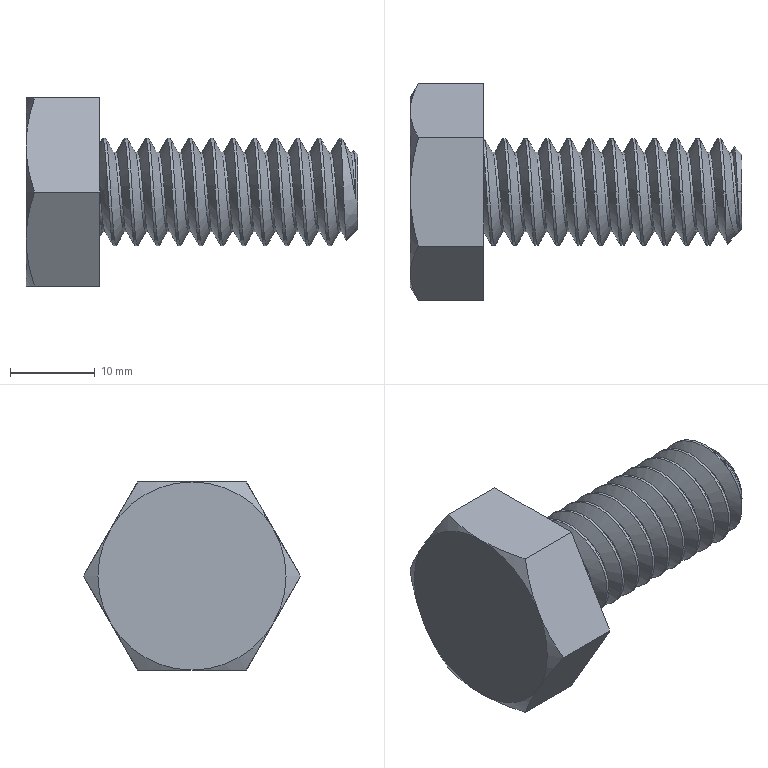Part | SolidWorks | features ICE 2, Chamfer 1, Extrusion 1, Helix 1, Revolution 1, Scale 1, SweepCut 1 | 1 solid | 44 faces | box 39.211 x 25.663 x 22.225 mm | volume 6651 mm3 | cylinder 24 | plane 9 | cone 8 | spline 3 | commonest cylinder face diameters 12.7 x24